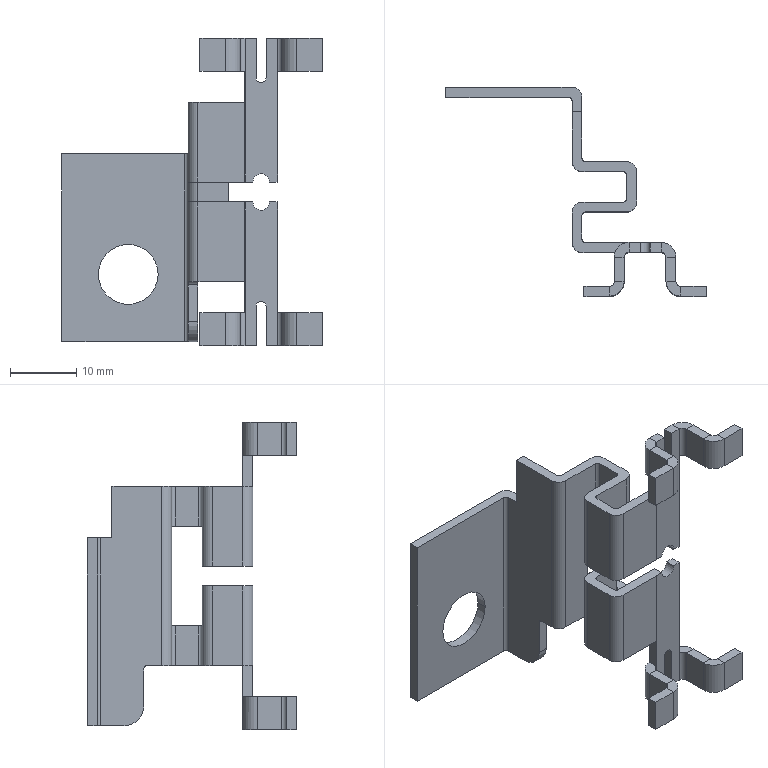Part | SolidWorks | features ICE 8, Fillet 4, FlatPattern 1, SMBaseFlange 1, SheetMetal 1 | 1 solid | 148 faces | box 39.2 x 31.5 x 46.3 mm | volume 2979 mm3 | plane 104 | cylinder 44 | commonest cylinder face diameters 1 x11 3 x10 1.473 x8 4.473 x8 1.5 x2 2.5 x2